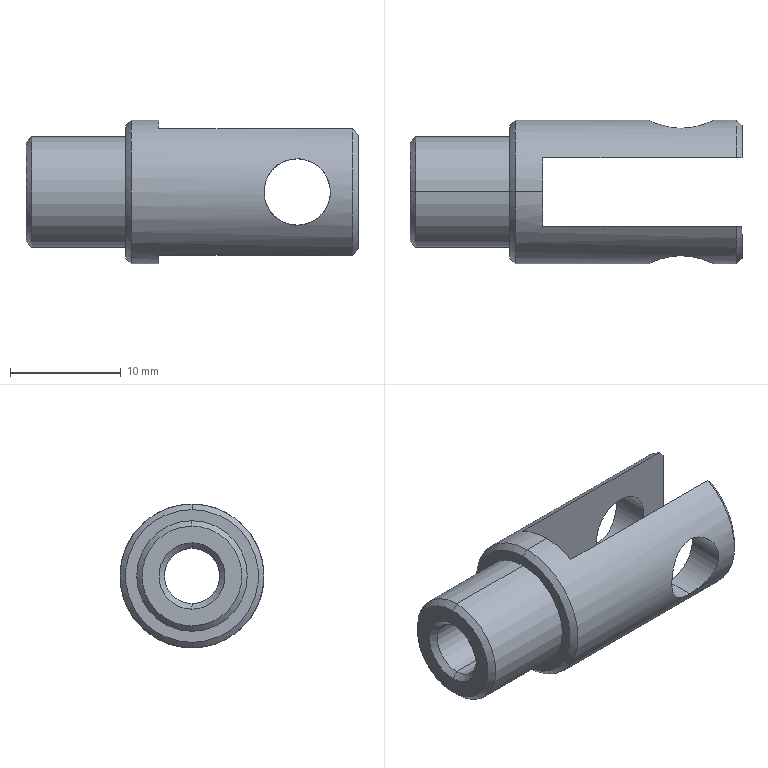Part | STEP file | 101000005929 | 1 solid | 25 faces | box 30 x 13 x 13 mm | volume 1668 mm3 | cylinder 10 | cone 8 | plane 7 | commonest cylinder face diameters 6 x4 5 x2 10 x2 13 x2
STEP:
#1=CARTESIAN_POINT('',(-29.5,0.,-2.5));
#2=VERTEX_POINT('',#1);
#3=CARTESIAN_POINT('',(-29.5,0.,2.5));
#4=VERTEX_POINT('',#3);
#5=CARTESIAN_POINT('',(-29.5,0.,0.));
#6=DIRECTION('',(-1.,0.,0.));
#7=AXIS2_PLACEMENT_3D('',#5,#6,$);
#8=CIRCLE('',#7,2.5);
#9=EDGE_CURVE('',#2,#4,#8,.T.);
#10=ORIENTED_EDGE('',*,*,#9,.F.);
#11=CARTESIAN_POINT('',(-30.,0.,-3.));
#12=VERTEX_POINT('',#11);
#13=CARTESIAN_POINT('',(-353581.641,0.,-353554.641));
#14=DIRECTION('',(-0.7071,0.,-0.7071));
#15=VECTOR('',#14,1.);
#16=LINE('',#13,#15);
#17=EDGE_CURVE('',#2,#12,#16,.T.);
#18=ORIENTED_EDGE('',*,*,#17,.T.);
#19=CARTESIAN_POINT('',(-30.,0.,3.));
#20=VERTEX_POINT('',#19);
#21=CARTESIAN_POINT('',(-30.,0.,0.));
#22=DIRECTION('',(-1.,0.,0.));
#23=AXIS2_PLACEMENT_3D('',#21,#22,$);
#24=CIRCLE('',#23,3.);
#25=EDGE_CURVE('',#20,#12,#24,.F.);
#26=ORIENTED_EDGE('',*,*,#25,.F.);
#27=CARTESIAN_POINT('',(-353581.641,0.,353554.641));
#28=DIRECTION('',(-0.7071,0.,0.7071));
#29=VECTOR('',#28,1.);
#30=LINE('',#27,#29);
#31=EDGE_CURVE('',#4,#20,#30,.T.);
#32=ORIENTED_EDGE('',*,*,#31,.F.);
#33=EDGE_LOOP('',(#10,#18,#26,#32));
#34=FACE_OUTER_BOUND('',#33,.T.);
#35=CARTESIAN_POINT('',(-29.5,0.,0.));
#36=DIRECTION('',(-1.,0.,0.));
#37=DIRECTION('',(0.,0.,-1.));
#38=AXIS2_PLACEMENT_3D('',#35,#36,#37);
#39=CONICAL_SURFACE('',#38,2.5,0.7854);
#40=ADVANCED_FACE('',(#34),#39,.F.);
#41=CARTESIAN_POINT('',(-18.,0.,2.5));
#42=VERTEX_POINT('',#41);
#43=CARTESIAN_POINT('',(-18.,0.,-2.5));
#44=VERTEX_POINT('',#43);
#45=CARTESIAN_POINT('',(-18.,0.,0.));
#46=DIRECTION('',(-1.,0.,0.));
#47=AXIS2_PLACEMENT_3D('',#45,#46,$);
#48=CIRCLE('',#47,2.5);
#49=EDGE_CURVE('',#42,#44,#48,.F.);
#50=ORIENTED_EDGE('',*,*,#49,.T.);
#51=CARTESIAN_POINT('',(-30.,0.,-2.5));
#52=DIRECTION('',(-1.,0.,0.));
#53=VECTOR('',#52,1.);
#54=LINE('',#51,#53);
#55=EDGE_CURVE('',#44,#2,#54,.T.);
#56=ORIENTED_EDGE('',*,*,#55,.T.);
#57=ORIENTED_EDGE('',*,*,#9,.T.);
#58=CARTESIAN_POINT('',(-30.,0.,2.5));
#59=DIRECTION('',(-1.,0.,0.));
#60=VECTOR('',#59,1.);
#61=LINE('',#58,#60);
#62=EDGE_CURVE('',#42,#4,#61,.T.);
#63=ORIENTED_EDGE('',*,*,#62,.F.);
#64=EDGE_LOOP('',(#50,#56,#57,#63));
#65=FACE_OUTER_BOUND('',#64,.T.);
#66=CARTESIAN_POINT('',(-30.,0.,0.));
#67=DIRECTION('',(-1.,0.,0.));
#68=DIRECTION('',(0.,0.,-1.));
#69=AXIS2_PLACEMENT_3D('',#66,#67,#68);
#70=CYLINDRICAL_SURFACE('',#69,2.5);
#71=ADVANCED_FACE('',(#65),#70,.F.);
#72=ORIENTED_EDGE('',*,*,#17,.F.);
#73=CARTESIAN_POINT('',(-29.5,0.,0.));
#74=DIRECTION('',(-1.,0.,0.));
#75=AXIS2_PLACEMENT_3D('',#73,#74,$);
#76=CIRCLE('',#75,2.5);
#77=EDGE_CURVE('',#4,#2,#76,.T.);
#78=ORIENTED_EDGE('',*,*,#77,.F.);
#79=ORIENTED_EDGE('',*,*,#31,.T.);
#80=CARTESIAN_POINT('',(-30.,0.,0.));
#81=DIRECTION('',(-1.,0.,0.));
#82=AXIS2_PLACEMENT_3D('',#80,#81,$);
#83=CIRCLE('',#82,3.);
#84=EDGE_CURVE('',#12,#20,#83,.F.);
#85=ORIENTED_EDGE('',*,*,#84,.F.);
#86=EDGE_LOOP('',(#72,#78,#79,#85));
#87=FACE_OUTER_BOUND('',#86,.T.);
#88=CARTESIAN_POINT('',(-29.5,0.,0.));
#89=DIRECTION('',(-1.,0.,0.));
#90=DIRECTION('',(0.,0.,1.));
#91=AXIS2_PLACEMENT_3D('',#88,#89,#90);
#92=CONICAL_SURFACE('',#91,2.5,0.7854);
#93=ADVANCED_FACE('',(#87),#92,.F.);
#94=CARTESIAN_POINT('',(-30.,0.,-4.5));
#95=VERTEX_POINT('',#94);
#96=CARTESIAN_POINT('',(-30.,0.,4.5));
#97=VERTEX_POINT('',#96);
#98=CARTESIAN_POINT('',(-30.,0.,-4.5));
#99=CARTESIAN_POINT('',(-30.,-0.4157,-4.5));
#100=CARTESIAN_POINT('',(-30.,-0.8314,-4.452));
#101=CARTESIAN_POINT('',(-30.,-1.24,-4.356));
#102=CARTESIAN_POINT('',(-30.,-2.027,-4.071));
#103=CARTESIAN_POINT('',(-30.,-2.728,-3.615));
#104=CARTESIAN_POINT('',(-30.,-3.051,-3.347));
#105=CARTESIAN_POINT('',(-30.,-3.629,-2.742));
#106=CARTESIAN_POINT('',(-30.,-4.053,-2.02));
#107=CARTESIAN_POINT('',(-30.,-4.223,-1.637));
#108=CARTESIAN_POINT('',(-30.,-4.47,-0.8373));
#109=CARTESIAN_POINT('',(-30.,-4.529,-0.002445));
#110=CARTESIAN_POINT('',(-30.,-4.51,0.4166));
#111=CARTESIAN_POINT('',(-30.,-4.375,1.243));
#112=CARTESIAN_POINT('',(-30.,-4.055,2.016));
#113=CARTESIAN_POINT('',(-30.,-3.852,2.383));
#114=CARTESIAN_POINT('',(-30.,-3.363,3.062));
#115=CARTESIAN_POINT('',(-30.,-2.732,3.612));
#116=CARTESIAN_POINT('',(-30.,-2.386,3.849));
#117=CARTESIAN_POINT('',(-30.,-1.719,4.201));
#118=CARTESIAN_POINT('',(-30.,-0.996,4.407));
#119=CARTESIAN_POINT('',(-30.,-0.6666,4.469));
#120=CARTESIAN_POINT('',(-30.,-0.3333,4.5));
#121=CARTESIAN_POINT('',(-30.,0.,4.5));
#122=B_SPLINE_CURVE_WITH_KNOTS('',5,(#98,#99,#100,#101,#102,#103,#104,#105,#106,#107,#108,#109,#110,#111,#112,#113,#114,#115,#116,#117,#118,#119,#120,#121),.UNSPECIFIED.,.F.,.U.,(6,3,3,3,3,3,3,6),(0.,2.939,5.879,8.818,11.757,14.697,17.636,19.993),.UNSPECIFIED.);
#123=EDGE_CURVE('',#95,#97,#122,.T.);
#124=ORIENTED_EDGE('',*,*,#123,.T.);
#125=CARTESIAN_POINT('',(-30.,0.,4.5));
#126=CARTESIAN_POINT('',(-30.,0.4157,4.5));
#127=CARTESIAN_POINT('',(-30.,0.8314,4.452));
#128=CARTESIAN_POINT('',(-30.,1.24,4.356));
#129=CARTESIAN_POINT('',(-30.,2.027,4.071));
#130=CARTESIAN_POINT('',(-30.,2.728,3.615));
#131=CARTESIAN_POINT('',(-30.,3.051,3.347));
#132=CARTESIAN_POINT('',(-30.,3.629,2.742));
#133=CARTESIAN_POINT('',(-30.,4.053,2.02));
#134=CARTESIAN_POINT('',(-30.,4.223,1.637));
#135=CARTESIAN_POINT('',(-30.,4.47,0.8373));
#136=CARTESIAN_POINT('',(-30.,4.529,0.002445));
#137=CARTESIAN_POINT('',(-30.,4.51,-0.4166));
#138=CARTESIAN_POINT('',(-30.,4.375,-1.243));
#139=CARTESIAN_POINT('',(-30.,4.055,-2.016));
#140=CARTESIAN_POINT('',(-30.,3.852,-2.383));
#141=CARTESIAN_POINT('',(-30.,3.363,-3.062));
#142=CARTESIAN_POINT('',(-30.,2.732,-3.612));
#143=CARTESIAN_POINT('',(-30.,2.386,-3.849));
#144=CARTESIAN_POINT('',(-30.,1.719,-4.201));
#145=CARTESIAN_POINT('',(-30.,0.996,-4.407));
#146=CARTESIAN_POINT('',(-30.,0.6666,-4.469));
#147=CARTESIAN_POINT('',(-30.,0.3333,-4.5));
#148=CARTESIAN_POINT('',(-30.,0.,-4.5));
#149=B_SPLINE_CURVE_WITH_KNOTS('',5,(#125,#126,#127,#128,#129,#130,#131,#132,#133,#134,#135,#136,#137,#138,#139,#140,#141,#142,#143,#144,#145,#146,#147,#148),.UNSPECIFIED.,.F.,.U.,(6,3,3,3,3,3,3,6),(0.,2.939,5.879,8.818,11.757,14.697,17.636,19.993),.UNSPECIFIED.);
#150=EDGE_CURVE('',#97,#95,#149,.T.);
#151=ORIENTED_EDGE('',*,*,#150,.T.);
#152=EDGE_LOOP('',(#124,#151));
#153=FACE_OUTER_BOUND('',#152,.T.);
#154=ORIENTED_EDGE('',*,*,#25,.T.);
#155=ORIENTED_EDGE('',*,*,#84,.T.);
#156=EDGE_LOOP('',(#154,#155));
#157=FACE_BOUND('',#156,.T.);
#158=CARTESIAN_POINT('',(-30.,0.,0.));
#159=DIRECTION('',(1.,0.,0.));
#160=DIRECTION('',(0.,0.,-1.));
#161=AXIS2_PLACEMENT_3D('',#158,#159,#160);
#162=PLANE('',#161);
#163=ADVANCED_FACE('',(#153,#157),#162,.F.);
#164=CARTESIAN_POINT('',(-18.,3.1,5.713));
#165=VERTEX_POINT('',#164);
#166=CARTESIAN_POINT('',(-18.,3.1,-5.713));
#167=VERTEX_POINT('',#166);
#168=CARTESIAN_POINT('',(-18.,3.1,0.));
#169=DIRECTION('',(0.,0.,-1.));
#170=VECTOR('',#169,1.);
#171=LINE('',#168,#170);
#172=EDGE_CURVE('',#165,#167,#171,.T.);
#173=ORIENTED_EDGE('',*,*,#172,.F.);
#174=CARTESIAN_POINT('',(-18.,0.,6.5));
#175=VERTEX_POINT('',#174);
#176=CARTESIAN_POINT('',(-18.,-0.000000001,0.000000005));
#177=DIRECTION('',(1.,0.,0.));
#178=AXIS2_PLACEMENT_3D('',#176,#177,$);
#179=CIRCLE('',#178,6.5);
#180=EDGE_CURVE('',#165,#175,#179,.T.);
#181=ORIENTED_EDGE('',*,*,#180,.T.);
#182=CARTESIAN_POINT('',(-18.,-3.1,5.713));
#183=VERTEX_POINT('',#182);
#184=CARTESIAN_POINT('',(-18.,0.000000002,0.000000005));
#185=DIRECTION('',(1.,0.,0.));
#186=AXIS2_PLACEMENT_3D('',#184,#185,$);
#187=CIRCLE('',#186,6.5);
#188=EDGE_CURVE('',#175,#183,#187,.T.);
#189=ORIENTED_EDGE('',*,*,#188,.T.);
#190=CARTESIAN_POINT('',(-18.,-3.1,-5.713));
#191=VERTEX_POINT('',#190);
#192=CARTESIAN_POINT('',(-18.,-3.1,0.));
#193=DIRECTION('',(0.,0.,-1.));
#194=VECTOR('',#193,1.);
#195=LINE('',#192,#194);
#196=EDGE_CURVE('',#183,#191,#195,.T.);
#197=ORIENTED_EDGE('',*,*,#196,.T.);
#198=CARTESIAN_POINT('',(-18.,0.,-6.5));
#199=VERTEX_POINT('',#198);
#200=CARTESIAN_POINT('',(-18.,-0.000000009,-0.000000034));
#201=DIRECTION('',(1.,0.,0.));
#202=AXIS2_PLACEMENT_3D('',#200,#201,$);
#203=CIRCLE('',#202,6.5);
#204=EDGE_CURVE('',#191,#199,#203,.T.);
#205=ORIENTED_EDGE('',*,*,#204,.T.);
#206=CARTESIAN_POINT('',(-18.,0.00000001,-0.000000034));
#207=DIRECTION('',(1.,0.,0.));
#208=AXIS2_PLACEMENT_3D('',#206,#207,$);
#209=CIRCLE('',#208,6.5);
#210=EDGE_CURVE('',#199,#167,#209,.T.);
#211=ORIENTED_EDGE('',*,*,#210,.T.);
#212=EDGE_LOOP('',(#173,#181,#189,#197,#205,#211));
#213=FACE_OUTER_BOUND('',#212,.T.);
#214=ORIENTED_EDGE('',*,*,#49,.F.);
#215=CARTESIAN_POINT('',(-18.,0.,0.000000001));
#216=DIRECTION('',(1.,0.,0.));
#217=AXIS2_PLACEMENT_3D('',#215,#216,$);
#218=CIRCLE('',#217,2.5);
#219=EDGE_CURVE('',#44,#42,#218,.T.);
#220=ORIENTED_EDGE('',*,*,#219,.F.);
#221=EDGE_LOOP('',(#214,#220));
#222=FACE_BOUND('',#221,.T.);
#223=CARTESIAN_POINT('',(-18.,3.1,50.232));
#224=DIRECTION('',(1.,0.,0.));
#225=DIRECTION('',(0.,1.,0.));
#226=AXIS2_PLACEMENT_3D('',#223,#224,#225);
#227=PLANE('',#226);
#228=ADVANCED_FACE('',(#213,#222),#227,.T.);
#229=ORIENTED_EDGE('',*,*,#55,.F.);
#230=ORIENTED_EDGE('',*,*,#219,.T.);
#231=ORIENTED_EDGE('',*,*,#62,.T.);
#232=ORIENTED_EDGE('',*,*,#77,.T.);
#233=EDGE_LOOP('',(#229,#230,#231,#232));
#234=FACE_OUTER_BOUND('',#233,.T.);
#235=CARTESIAN_POINT('',(-30.,0.,0.));
#236=DIRECTION('',(-1.,0.,0.));
#237=DIRECTION('',(0.,0.,1.));
#238=AXIS2_PLACEMENT_3D('',#235,#236,#237);
#239=CYLINDRICAL_SURFACE('',#238,2.5);
#240=ADVANCED_FACE('',(#234),#239,.F.);
#241=CARTESIAN_POINT('',(-29.5,0.,5.));
#242=VERTEX_POINT('',#241);
#243=CARTESIAN_POINT('',(353521.141,0.,353555.641));
#244=DIRECTION('',(0.7071,0.,0.7071));
#245=VECTOR('',#244,1.);
#246=LINE('',#243,#245);
#247=EDGE_CURVE('',#97,#242,#246,.T.);
#248=ORIENTED_EDGE('',*,*,#247,.F.);
#249=ORIENTED_EDGE('',*,*,#123,.F.);
#250=CARTESIAN_POINT('',(-29.5,0.,-5.));
#251=VERTEX_POINT('',#250);
#252=CARTESIAN_POINT('',(353521.141,0.,-353555.641));
#253=DIRECTION('',(0.7071,0.,-0.7071));
#254=VECTOR('',#253,1.);
#255=LINE('',#252,#254);
#256=EDGE_CURVE('',#95,#251,#255,.T.);
#257=ORIENTED_EDGE('',*,*,#256,.T.);
#258=CARTESIAN_POINT('',(-29.5,0.,0.));
#259=DIRECTION('',(1.,0.,0.));
#260=AXIS2_PLACEMENT_3D('',#258,#259,$);
#261=CIRCLE('',#260,5.);
#262=EDGE_CURVE('',#242,#251,#261,.T.);
#263=ORIENTED_EDGE('',*,*,#262,.F.);
#264=EDGE_LOOP('',(#248,#249,#257,#263));
#265=FACE_OUTER_BOUND('',#264,.T.);
#266=CARTESIAN_POINT('',(-30.,0.,0.));
#267=DIRECTION('',(1.,0.,0.));
#268=DIRECTION('',(0.,0.,1.));
#269=AXIS2_PLACEMENT_3D('',#266,#267,#268);
#270=CONICAL_SURFACE('',#269,4.5,0.7854);
#271=ADVANCED_FACE('',(#265),#270,.T.);
#272=ORIENTED_EDGE('',*,*,#150,.F.);
#273=ORIENTED_EDGE('',*,*,#247,.T.);
#274=CARTESIAN_POINT('',(-29.5,0.,0.));
#275=DIRECTION('',(1.,0.,0.));
#276=AXIS2_PLACEMENT_3D('',#274,#275,$);
#277=CIRCLE('',#276,5.);
#278=EDGE_CURVE('',#251,#242,#277,.T.);
#279=ORIENTED_EDGE('',*,*,#278,.F.);
#280=ORIENTED_EDGE('',*,*,#256,.F.);
#281=EDGE_LOOP('',(#272,#273,#279,#280));
#282=FACE_OUTER_BOUND('',#281,.T.);
#283=CARTESIAN_POINT('',(-30.,0.,0.));
#284=DIRECTION('',(1.,0.,0.));
#285=DIRECTION('',(0.,0.,-1.));
#286=AXIS2_PLACEMENT_3D('',#283,#284,#285);
#287=CONICAL_SURFACE('',#286,4.5,0.7854);
#288=ADVANCED_FACE('',(#282),#287,.T.);
#289=CARTESIAN_POINT('',(-0.5,3.1,-5.713));
#290=VERTEX_POINT('',#289);
#291=CARTESIAN_POINT('',(-9.25,3.1,-5.713));
#292=DIRECTION('',(1.,0.,0.));
#293=VECTOR('',#292,1.);
#294=LINE('',#291,#293);
#295=EDGE_CURVE('',#167,#290,#294,.T.);
#296=ORIENTED_EDGE('',*,*,#295,.T.);
#297=CARTESIAN_POINT('',(0.,3.1,-5.137));
#298=VERTEX_POINT('',#297);
#299=CARTESIAN_POINT('',(-0.5,3.1,-5.713));
#300=CARTESIAN_POINT('',(-0.3993,3.1,-5.599));
#301=CARTESIAN_POINT('',(-0.2989,3.1,-5.484));
#302=CARTESIAN_POINT('',(-0.1989,3.1,-5.369));
#303=CARTESIAN_POINT('',(-0.09922,3.1,-5.253));
#304=CARTESIAN_POINT('',(0.,3.1,-5.137));
#305=B_SPLINE_CURVE_WITH_KNOTS('',5,(#299,#300,#301,#302,#303,#304),.UNSPECIFIED.,.F.,.U.,(6,6),(0.,1.079),.UNSPECIFIED.);
#306=EDGE_CURVE('',#290,#298,#305,.T.);
#307=ORIENTED_EDGE('',*,*,#306,.T.);
#308=CARTESIAN_POINT('',(0.,3.1,5.137));
#309=VERTEX_POINT('',#308);
#310=CARTESIAN_POINT('',(0.,3.1,0.));
#311=DIRECTION('',(0.,0.,1.));
#312=VECTOR('',#311,1.);
#313=LINE('',#310,#312);
#314=EDGE_CURVE('',#298,#309,#313,.T.);
#315=ORIENTED_EDGE('',*,*,#314,.T.);
#316=CARTESIAN_POINT('',(-0.5,3.1,5.713));
#317=VERTEX_POINT('',#316);
#318=CARTESIAN_POINT('',(0.,3.1,5.137));
#319=CARTESIAN_POINT('',(-0.09922,3.1,5.253));
#320=CARTESIAN_POINT('',(-0.1989,3.1,5.369));
#321=CARTESIAN_POINT('',(-0.2989,3.1,5.484));
#322=CARTESIAN_POINT('',(-0.3993,3.1,5.599));
#323=CARTESIAN_POINT('',(-0.5,3.1,5.713));
#324=B_SPLINE_CURVE_WITH_KNOTS('',5,(#318,#319,#320,#321,#322,#323),.UNSPECIFIED.,.F.,.U.,(6,6),(0.,1.079),.UNSPECIFIED.);
#325=EDGE_CURVE('',#309,#317,#324,.T.);
#326=ORIENTED_EDGE('',*,*,#325,.T.);
#327=CARTESIAN_POINT('',(-9.25,3.1,5.713));
#328=DIRECTION('',(-1.,0.,0.));
#329=VECTOR('',#328,1.);
#330=LINE('',#327,#329);
#331=EDGE_CURVE('',#317,#165,#330,.T.);
#332=ORIENTED_EDGE('',*,*,#331,.T.);
#333=ORIENTED_EDGE('',*,*,#172,.T.);
#334=EDGE_LOOP('',(#296,#307,#315,#326,#332,#333));
#335=FACE_OUTER_BOUND('',#334,.T.);
#336=CARTESIAN_POINT('',(-5.5,3.1,-3.));
#337=VERTEX_POINT('',#336);
#338=CARTESIAN_POINT('',(-5.5,3.1,3.));
#339=VERTEX_POINT('',#338);
#340=CARTESIAN_POINT('',(-5.5,3.1,-3.));
#341=CARTESIAN_POINT('',(-5.839,3.1,-3.));
#342=CARTESIAN_POINT('',(-6.179,3.1,-2.952));
#343=CARTESIAN_POINT('',(-6.509,3.1,-2.856));
#344=CARTESIAN_POINT('',(-7.134,3.1,-2.573));
#345=CARTESIAN_POINT('',(-7.655,3.1,-2.128));
#346=CARTESIAN_POINT('',(-7.883,3.1,-1.87));
#347=CARTESIAN_POINT('',(-8.258,3.1,-1.297));
#348=CARTESIAN_POINT('',(-8.46,3.1,-0.6415));
#349=CARTESIAN_POINT('',(-8.514,3.1,-0.3017));
#350=CARTESIAN_POINT('',(-8.524,3.1,0.3838));
#351=CARTESIAN_POINT('',(-8.343,3.1,1.045));
#352=CARTESIAN_POINT('',(-8.206,3.1,1.361));
#353=CARTESIAN_POINT('',(-7.847,3.1,1.945));
#354=CARTESIAN_POINT('',(-7.34,3.1,2.406));
#355=CARTESIAN_POINT('',(-7.055,3.1,2.599));
#356=CARTESIAN_POINT('',(-6.577,3.1,2.833));
#357=CARTESIAN_POINT('',(-6.062,3.1,2.956));
#358=CARTESIAN_POINT('',(-5.876,3.1,2.985));
#359=CARTESIAN_POINT('',(-5.688,3.1,3.));
#360=CARTESIAN_POINT('',(-5.5,3.1,3.));
#361=B_SPLINE_CURVE_WITH_KNOTS('',5,(#340,#341,#342,#343,#344,#345,#346,#347,#348,#349,#350,#351,#352,#353,#354,#355,#356,#357,#358,#359,#360),.UNSPECIFIED.,.F.,.U.,(6,3,3,3,3,3,6),(0.,2.4,4.8,7.2,9.6,12.,13.328),.UNSPECIFIED.);
#362=EDGE_CURVE('',#337,#339,#361,.T.);
#363=ORIENTED_EDGE('',*,*,#362,.T.);
#364=CARTESIAN_POINT('',(-5.5,3.1,3.));
#365=CARTESIAN_POINT('',(-5.161,3.1,3.));
#366=CARTESIAN_POINT('',(-4.821,3.1,2.952));
#367=CARTESIAN_POINT('',(-4.491,3.1,2.856));
#368=CARTESIAN_POINT('',(-3.866,3.1,2.573));
#369=CARTESIAN_POINT('',(-3.345,3.1,2.128));
#370=CARTESIAN_POINT('',(-3.117,3.1,1.87));
#371=CARTESIAN_POINT('',(-2.742,3.1,1.297));
#372=CARTESIAN_POINT('',(-2.54,3.1,0.6415));
#373=CARTESIAN_POINT('',(-2.486,3.1,0.3017));
#374=CARTESIAN_POINT('',(-2.476,3.1,-0.3838));
#375=CARTESIAN_POINT('',(-2.657,3.1,-1.045));
#376=CARTESIAN_POINT('',(-2.794,3.1,-1.361));
#377=CARTESIAN_POINT('',(-3.153,3.1,-1.945));
#378=CARTESIAN_POINT('',(-3.66,3.1,-2.406));
#379=CARTESIAN_POINT('',(-3.945,3.1,-2.599));
#380=CARTESIAN_POINT('',(-4.423,3.1,-2.833));
#381=CARTESIAN_POINT('',(-4.938,3.1,-2.956));
#382=CARTESIAN_POINT('',(-5.124,3.1,-2.985));
#383=CARTESIAN_POINT('',(-5.312,3.1,-3.));
#384=CARTESIAN_POINT('',(-5.5,3.1,-3.));
#385=B_SPLINE_CURVE_WITH_KNOTS('',5,(#364,#365,#366,#367,#368,#369,#370,#371,#372,#373,#374,#375,#376,#377,#378,#379,#380,#381,#382,#383,#384),.UNSPECIFIED.,.F.,.U.,(6,3,3,3,3,3,6),(0.,2.4,4.8,7.2,9.6,12.,13.328),.UNSPECIFIED.);
#386=EDGE_CURVE('',#339,#337,#385,.T.);
#387=ORIENTED_EDGE('',*,*,#386,.T.);
#388=EDGE_LOOP('',(#363,#387));
#389=FACE_BOUND('',#388,.T.);
#390=CARTESIAN_POINT('',(0.,3.1,50.232));
#391=DIRECTION('',(0.,-1.,0.));
#392=DIRECTION('',(1.,0.,0.));
#393=AXIS2_PLACEMENT_3D('',#390,#391,#392);
#394=PLANE('',#393);
#395=ADVANCED_FACE('',(#335,#389),#394,.T.);
#396=ORIENTED_EDGE('',*,*,#210,.F.);
#397=CARTESIAN_POINT('',(-20.5,0.,-6.5));
#398=VERTEX_POINT('',#397);
#399=CARTESIAN_POINT('',(-30.,0.,-6.5));
#400=DIRECTION('',(-1.,0.,0.));
#401=VECTOR('',#400,1.);
#402=LINE('',#399,#401);
#403=EDGE_CURVE('',#199,#398,#402,.T.);
#404=ORIENTED_EDGE('',*,*,#403,.T.);
#405=CARTESIAN_POINT('',(-20.5,0.,6.5));
#406=VERTEX_POINT('',#405);
#407=CARTESIAN_POINT('',(-20.5,0.,0.));
#408=DIRECTION('',(-1.,0.,0.));
#409=AXIS2_PLACEMENT_3D('',#407,#408,$);
#410=CIRCLE('',#409,6.5);
#411=EDGE_CURVE('',#398,#406,#410,.F.);
#412=ORIENTED_EDGE('',*,*,#411,.T.);
#413=CARTESIAN_POINT('',(-30.,0.,6.5));
#414=DIRECTION('',(-1.,0.,0.));
#415=VECTOR('',#414,1.);
#416=LINE('',#413,#415);
#417=EDGE_CURVE('',#175,#406,#416,.T.);
#418=ORIENTED_EDGE('',*,*,#417,.F.);
#419=ORIENTED_EDGE('',*,*,#180,.F.);
#420=ORIENTED_EDGE('',*,*,#331,.F.);
#421=CARTESIAN_POINT('',(-0.5,0.,0.));
#422=DIRECTION('',(-1.,0.,0.));
#423=AXIS2_PLACEMENT_3D('',#421,#422,$);
#424=CIRCLE('',#423,6.5);
#425=EDGE_CURVE('',#317,#290,#424,.T.);
#426=ORIENTED_EDGE('',*,*,#425,.T.);
#427=ORIENTED_EDGE('',*,*,#295,.F.);
#428=EDGE_LOOP('',(#396,#404,#412,#418,#419,#420,#426,#427));
#429=FACE_OUTER_BOUND('',#428,.T.);
#430=CARTESIAN_POINT('',(-5.5,5.766,-3.));
#431=VERTEX_POINT('',#430);
#432=CARTESIAN_POINT('',(-5.5,5.766,3.));
#433=VERTEX_POINT('',#432);
#434=CARTESIAN_POINT('',(-5.5,5.766,-3.));
#435=CARTESIAN_POINT('',(-5.829,5.766,-3.));
#436=CARTESIAN_POINT('',(-6.152,5.789,-2.956));
#437=CARTESIAN_POINT('',(-6.469,5.835,-2.867));
#438=CARTESIAN_POINT('',(-7.002,5.947,-2.636));
#439=CARTESIAN_POINT('',(-7.461,6.086,-2.291));
#440=CARTESIAN_POINT('',(-7.645,6.149,-2.121));
#441=CARTESIAN_POINT('',(-8.024,6.29,-1.684));
#442=CARTESIAN_POINT('',(-8.293,6.405,-1.167));
#443=CARTESIAN_POINT('',(-8.404,6.456,-0.8542));
#444=CARTESIAN_POINT('',(-8.538,6.517,-0.2095));
#445=CARTESIAN_POINT('',(-8.493,6.497,0.4514));
#446=CARTESIAN_POINT('',(-8.425,6.465,0.7775));
#447=CARTESIAN_POINT('',(-8.229,6.377,1.326));
#448=CARTESIAN_POINT('',(-7.916,6.25,1.805));
#449=CARTESIAN_POINT('',(-7.755,6.188,2.002));
#450=CARTESIAN_POINT('',(-7.46,6.085,2.296));
#451=CARTESIAN_POINT('',(-7.118,5.987,2.534));
#452=CARTESIAN_POINT('',(-6.974,5.949,2.621));
#453=CARTESIAN_POINT('',(-6.614,5.866,2.805));
#454=CARTESIAN_POINT('',(-6.223,5.805,2.926));
#455=CARTESIAN_POINT('',(-5.984,5.779,2.975));
#456=CARTESIAN_POINT('',(-5.741,5.766,3.));
#457=CARTESIAN_POINT('',(-5.5,5.766,3.));
#458=B_SPLINE_CURVE_WITH_KNOTS('',5,(#434,#435,#436,#437,#438,#439,#440,#441,#442,#443,#444,#445,#446,#447,#448,#449,#450,#451,#452,#453,#454,#455,#456,#457),.UNSPECIFIED.,.F.,.U.,(6,3,3,3,3,3,3,6),(0.,2.313,4.158,6.496,8.8,10.625,11.825,13.541),.UNSPECIFIED.);
#459=EDGE_CURVE('',#431,#433,#458,.T.);
#460=ORIENTED_EDGE('',*,*,#459,.F.);
#461=CARTESIAN_POINT('',(-5.5,5.766,3.));
#462=CARTESIAN_POINT('',(-5.089,5.766,3.));
#463=CARTESIAN_POINT('',(-4.674,5.804,2.928));
#464=CARTESIAN_POINT('',(-4.284,5.877,2.788));
#465=CARTESIAN_POINT('',(-3.78,6.008,2.503));
#466=CARTESIAN_POINT('',(-3.363,6.148,2.115));
#467=CARTESIAN_POINT('',(-3.248,6.189,1.992));
#468=CARTESIAN_POINT('',(-3.039,6.268,1.735));
#469=CARTESIAN_POINT('',(-2.866,6.339,1.449));
#470=CARTESIAN_POINT('',(-2.789,6.371,1.301));
#471=CARTESIAN_POINT('',(-2.66,6.427,1.001));
#472=CARTESIAN_POINT('',(-2.573,6.467,0.6849));
#473=CARTESIAN_POINT('',(-2.54,6.482,0.5261));
#474=CARTESIAN_POINT('',(-2.485,6.507,0.1234));
#475=CARTESIAN_POINT('',(-2.498,6.501,-0.285));
#476=CARTESIAN_POINT('',(-2.532,6.485,-0.5294));
#477=CARTESIAN_POINT('',(-2.67,6.422,-1.097));
#478=CARTESIAN_POINT('',(-2.936,6.308,-1.612));
#479=CARTESIAN_POINT('',(-3.131,6.23,-1.884));
#480=CARTESIAN_POINT('',(-3.635,6.045,-2.421));
#481=CARTESIAN_POINT('',(-4.284,5.877,-2.787));
#482=CARTESIAN_POINT('',(-4.673,5.804,-2.928));
#483=CARTESIAN_POINT('',(-5.085,5.766,-3.));
#484=CARTESIAN_POINT('',(-5.5,5.766,-3.));
#485=B_SPLINE_CURVE_WITH_KNOTS('',5,(#461,#462,#463,#464,#465,#466,#467,#468,#469,#470,#471,#472,#473,#474,#475,#476,#477,#478,#479,#480,#481,#482,#483,#484),.UNSPECIFIED.,.F.,.U.,(6,3,3,3,3,3,3,6),(0.,2.915,4.139,5.326,6.479,8.198,10.612,13.532),.UNSPECIFIED.);
#486=EDGE_CURVE('',#433,#431,#485,.T.);
#487=ORIENTED_EDGE('',*,*,#486,.F.);
#488=EDGE_LOOP('',(#460,#487));
#489=FACE_BOUND('',#488,.T.);
#490=CARTESIAN_POINT('',(-30.,0.,0.));
#491=DIRECTION('',(-1.,0.,0.));
#492=DIRECTION('',(0.,0.,1.));
#493=AXIS2_PLACEMENT_3D('',#490,#491,#492);
#494=CYLINDRICAL_SURFACE('',#493,6.5);
#495=ADVANCED_FACE('',(#429,#489),#494,.T.);
#496=ORIENTED_EDGE('',*,*,#403,.F.);
#497=ORIENTED_EDGE('',*,*,#204,.F.);
#498=CARTESIAN_POINT('',(-0.5,-3.1,-5.713));
#499=VERTEX_POINT('',#498);
#500=CARTESIAN_POINT('',(-30.,-3.1,-5.713));
#501=DIRECTION('',(-1.,0.,0.));
#502=VECTOR('',#501,1.);
#503=LINE('',#500,#502);
#504=EDGE_CURVE('',#499,#191,#503,.T.);
#505=ORIENTED_EDGE('',*,*,#504,.F.);
#506=CARTESIAN_POINT('',(-0.5,-3.1,5.713));
#507=VERTEX_POINT('',#506);
#508=CARTESIAN_POINT('',(-0.5,0.,0.));
#509=DIRECTION('',(-1.,0.,0.));
#510=AXIS2_PLACEMENT_3D('',#508,#509,$);
#511=CIRCLE('',#510,6.5);
#512=EDGE_CURVE('',#499,#507,#511,.T.);
#513=ORIENTED_EDGE('',*,*,#512,.T.);
#514=CARTESIAN_POINT('',(-30.,-3.1,5.713));
#515=DIRECTION('',(-1.,0.,0.));
#516=VECTOR('',#515,1.);
#517=LINE('',#514,#516);
#518=EDGE_CURVE('',#183,#507,#517,.F.);
#519=ORIENTED_EDGE('',*,*,#518,.F.);
#520=ORIENTED_EDGE('',*,*,#188,.F.);
#521=ORIENTED_EDGE('',*,*,#417,.T.);
#522=CARTESIAN_POINT('',(-20.5,0.,0.));
#523=DIRECTION('',(-1.,0.,0.));
#524=AXIS2_PLACEMENT_3D('',#522,#523,$);
#525=CIRCLE('',#524,6.5);
#526=EDGE_CURVE('',#406,#398,#525,.F.);
#527=ORIENTED_EDGE('',*,*,#526,.T.);
#528=EDGE_LOOP('',(#496,#497,#505,#513,#519,#520,#521,#527));
#529=FACE_OUTER_BOUND('',#528,.T.);
#530=CARTESIAN_POINT('',(-5.5,-5.766,-3.));
#531=VERTEX_POINT('',#530);
#532=CARTESIAN_POINT('',(-5.5,-5.766,3.));
#533=VERTEX_POINT('',#532);
#534=CARTESIAN_POINT('',(-5.5,-5.766,-3.));
#535=CARTESIAN_POINT('',(-5.171,-5.766,-3.));
#536=CARTESIAN_POINT('',(-4.848,-5.789,-2.956));
#537=CARTESIAN_POINT('',(-4.531,-5.835,-2.867));
#538=CARTESIAN_POINT('',(-3.998,-5.947,-2.636));
#539=CARTESIAN_POINT('',(-3.539,-6.086,-2.291));
#540=CARTESIAN_POINT('',(-3.355,-6.149,-2.121));
#541=CARTESIAN_POINT('',(-2.976,-6.29,-1.684));
#542=CARTESIAN_POINT('',(-2.707,-6.405,-1.167));
#543=CARTESIAN_POINT('',(-2.596,-6.456,-0.8542));
#544=CARTESIAN_POINT('',(-2.462,-6.517,-0.2095));
#545=CARTESIAN_POINT('',(-2.507,-6.497,0.4514));
#546=CARTESIAN_POINT('',(-2.575,-6.465,0.7775));
#547=CARTESIAN_POINT('',(-2.771,-6.377,1.326));
#548=CARTESIAN_POINT('',(-3.084,-6.25,1.805));
#549=CARTESIAN_POINT('',(-3.245,-6.188,2.002));
#550=CARTESIAN_POINT('',(-3.54,-6.085,2.296));
#551=CARTESIAN_POINT('',(-3.882,-5.987,2.534));
#552=CARTESIAN_POINT('',(-4.026,-5.949,2.621));
#553=CARTESIAN_POINT('',(-4.386,-5.866,2.805));
#554=CARTESIAN_POINT('',(-4.777,-5.805,2.926));
#555=CARTESIAN_POINT('',(-5.016,-5.779,2.975));
#556=CARTESIAN_POINT('',(-5.259,-5.766,3.));
#557=CARTESIAN_POINT('',(-5.5,-5.766,3.));
#558=B_SPLINE_CURVE_WITH_KNOTS('',5,(#534,#535,#536,#537,#538,#539,#540,#541,#542,#543,#544,#545,#546,#547,#548,#549,#550,#551,#552,#553,#554,#555,#556,#557),.UNSPECIFIED.,.F.,.U.,(6,3,3,3,3,3,3,6),(0.,2.313,4.158,6.496,8.8,10.625,11.825,13.541),.UNSPECIFIED.);
#559=EDGE_CURVE('',#531,#533,#558,.T.);
#560=ORIENTED_EDGE('',*,*,#559,.F.);
#561=CARTESIAN_POINT('',(-5.5,-5.766,3.));
#562=CARTESIAN_POINT('',(-5.911,-5.766,3.));
#563=CARTESIAN_POINT('',(-6.326,-5.804,2.928));
#564=CARTESIAN_POINT('',(-6.716,-5.877,2.788));
#565=CARTESIAN_POINT('',(-7.22,-6.008,2.503));
#566=CARTESIAN_POINT('',(-7.637,-6.148,2.115));
#567=CARTESIAN_POINT('',(-7.752,-6.189,1.992));
#568=CARTESIAN_POINT('',(-7.961,-6.268,1.735));
#569=CARTESIAN_POINT('',(-8.134,-6.339,1.449));
#570=CARTESIAN_POINT('',(-8.211,-6.371,1.301));
#571=CARTESIAN_POINT('',(-8.34,-6.427,1.001));
#572=CARTESIAN_POINT('',(-8.427,-6.467,0.6849));
#573=CARTESIAN_POINT('',(-8.46,-6.482,0.5261));
#574=CARTESIAN_POINT('',(-8.515,-6.507,0.1234));
#575=CARTESIAN_POINT('',(-8.502,-6.501,-0.285));
#576=CARTESIAN_POINT('',(-8.468,-6.485,-0.5294));
#577=CARTESIAN_POINT('',(-8.33,-6.422,-1.097));
#578=CARTESIAN_POINT('',(-8.064,-6.308,-1.612));
#579=CARTESIAN_POINT('',(-7.869,-6.23,-1.884));
#580=CARTESIAN_POINT('',(-7.365,-6.045,-2.421));
#581=CARTESIAN_POINT('',(-6.716,-5.877,-2.787));
#582=CARTESIAN_POINT('',(-6.327,-5.804,-2.928));
#583=CARTESIAN_POINT('',(-5.915,-5.766,-3.));
#584=CARTESIAN_POINT('',(-5.5,-5.766,-3.));
#585=B_SPLINE_CURVE_WITH_KNOTS('',5,(#561,#562,#563,#564,#565,#566,#567,#568,#569,#570,#571,#572,#573,#574,#575,#576,#577,#578,#579,#580,#581,#582,#583,#584),.UNSPECIFIED.,.F.,.U.,(6,3,3,3,3,3,3,6),(0.,2.915,4.139,5.326,6.479,8.198,10.612,13.532),.UNSPECIFIED.);
#586=EDGE_CURVE('',#533,#531,#585,.T.);
#587=ORIENTED_EDGE('',*,*,#586,.F.);
#588=EDGE_LOOP('',(#560,#587));
#589=FACE_BOUND('',#588,.T.);
#590=CARTESIAN_POINT('',(-30.,0.,0.));
#591=DIRECTION('',(-1.,0.,0.));
#592=DIRECTION('',(0.,0.,-1.));
#593=AXIS2_PLACEMENT_3D('',#590,#591,#592);
#594=CYLINDRICAL_SURFACE('',#593,6.5);
#595=ADVANCED_FACE('',(#529,#589),#594,.T.);
#596=ORIENTED_EDGE('',*,*,#518,.T.);
#597=CARTESIAN_POINT('',(0.,-3.1,5.137));
#598=VERTEX_POINT('',#597);
#599=CARTESIAN_POINT('',(-0.5,-3.1,5.713));
#600=CARTESIAN_POINT('',(-0.3993,-3.1,5.599));
#601=CARTESIAN_POINT('',(-0.2989,-3.1,5.484));
#602=CARTESIAN_POINT('',(-0.1989,-3.1,5.369));
#603=CARTESIAN_POINT('',(-0.09922,-3.1,5.253));
#604=CARTESIAN_POINT('',(0.,-3.1,5.137));
#605=B_SPLINE_CURVE_WITH_KNOTS('',5,(#599,#600,#601,#602,#603,#604),.UNSPECIFIED.,.F.,.U.,(6,6),(0.,1.079),.UNSPECIFIED.);
#606=EDGE_CURVE('',#507,#598,#605,.T.);
#607=ORIENTED_EDGE('',*,*,#606,.T.);
#608=CARTESIAN_POINT('',(0.,-3.1,-5.137));
#609=VERTEX_POINT('',#608);
#610=CARTESIAN_POINT('',(0.,-3.1,0.));
#611=DIRECTION('',(0.,0.,-1.));
#612=VECTOR('',#611,1.);
#613=LINE('',#610,#612);
#614=EDGE_CURVE('',#598,#609,#613,.T.);
#615=ORIENTED_EDGE('',*,*,#614,.T.);
#616=CARTESIAN_POINT('',(0.,-3.1,-5.137));
#617=CARTESIAN_POINT('',(-0.09922,-3.1,-5.253));
#618=CARTESIAN_POINT('',(-0.1989,-3.1,-5.369));
#619=CARTESIAN_POINT('',(-0.2989,-3.1,-5.484));
#620=CARTESIAN_POINT('',(-0.3993,-3.1,-5.599));
#621=CARTESIAN_POINT('',(-0.5,-3.1,-5.713));
#622=B_SPLINE_CURVE_WITH_KNOTS('',5,(#616,#617,#618,#619,#620,#621),.UNSPECIFIED.,.F.,.U.,(6,6),(0.,1.079),.UNSPECIFIED.);
#623=EDGE_CURVE('',#609,#499,#622,.T.);
#624=ORIENTED_EDGE('',*,*,#623,.T.);
#625=ORIENTED_EDGE('',*,*,#504,.T.);
#626=ORIENTED_EDGE('',*,*,#196,.F.);
#627=EDGE_LOOP('',(#596,#607,#615,#624,#625,#626));
#628=FACE_OUTER_BOUND('',#627,.T.);
#629=CARTESIAN_POINT('',(-5.5,-3.1,-3.));
#630=VERTEX_POINT('',#629);
#631=CARTESIAN_POINT('',(-5.5,-3.1,3.));
#632=VERTEX_POINT('',#631);
#633=CARTESIAN_POINT('',(-5.5,-3.1,-3.));
#634=CARTESIAN_POINT('',(-5.161,-3.1,-3.));
#635=CARTESIAN_POINT('',(-4.821,-3.1,-2.952));
#636=CARTESIAN_POINT('',(-4.491,-3.1,-2.856));
#637=CARTESIAN_POINT('',(-3.866,-3.1,-2.573));
#638=CARTESIAN_POINT('',(-3.345,-3.1,-2.128));
#639=CARTESIAN_POINT('',(-3.117,-3.1,-1.87));
#640=CARTESIAN_POINT('',(-2.742,-3.1,-1.297));
#641=CARTESIAN_POINT('',(-2.54,-3.1,-0.6415));
#642=CARTESIAN_POINT('',(-2.486,-3.1,-0.3017));
#643=CARTESIAN_POINT('',(-2.476,-3.1,0.3838));
#644=CARTESIAN_POINT('',(-2.657,-3.1,1.045));
#645=CARTESIAN_POINT('',(-2.794,-3.1,1.361));
#646=CARTESIAN_POINT('',(-3.153,-3.1,1.945));
#647=CARTESIAN_POINT('',(-3.66,-3.1,2.406));
#648=CARTESIAN_POINT('',(-3.945,-3.1,2.599));
#649=CARTESIAN_POINT('',(-4.423,-3.1,2.833));
#650=CARTESIAN_POINT('',(-4.938,-3.1,2.956));
#651=CARTESIAN_POINT('',(-5.124,-3.1,2.985));
#652=CARTESIAN_POINT('',(-5.312,-3.1,3.));
#653=CARTESIAN_POINT('',(-5.5,-3.1,3.));
#654=B_SPLINE_CURVE_WITH_KNOTS('',5,(#633,#634,#635,#636,#637,#638,#639,#640,#641,#642,#643,#644,#645,#646,#647,#648,#649,#650,#651,#652,#653),.UNSPECIFIED.,.F.,.U.,(6,3,3,3,3,3,6),(0.,2.4,4.8,7.2,9.6,12.,13.328),.UNSPECIFIED.);
#655=EDGE_CURVE('',#630,#632,#654,.T.);
#656=ORIENTED_EDGE('',*,*,#655,.T.);
#657=CARTESIAN_POINT('',(-5.5,-3.1,3.));
#658=CARTESIAN_POINT('',(-5.839,-3.1,3.));
#659=CARTESIAN_POINT('',(-6.179,-3.1,2.952));
#660=CARTESIAN_POINT('',(-6.509,-3.1,2.856));
#661=CARTESIAN_POINT('',(-7.134,-3.1,2.573));
#662=CARTESIAN_POINT('',(-7.655,-3.1,2.128));
#663=CARTESIAN_POINT('',(-7.883,-3.1,1.87));
#664=CARTESIAN_POINT('',(-8.258,-3.1,1.297));
#665=CARTESIAN_POINT('',(-8.46,-3.1,0.6415));
#666=CARTESIAN_POINT('',(-8.514,-3.1,0.3017));
#667=CARTESIAN_POINT('',(-8.524,-3.1,-0.3838));
#668=CARTESIAN_POINT('',(-8.343,-3.1,-1.045));
#669=CARTESIAN_POINT('',(-8.206,-3.1,-1.361));
#670=CARTESIAN_POINT('',(-7.847,-3.1,-1.945));
#671=CARTESIAN_POINT('',(-7.34,-3.1,-2.406));
#672=CARTESIAN_POINT('',(-7.055,-3.1,-2.599));
#673=CARTESIAN_POINT('',(-6.577,-3.1,-2.833));
#674=CARTESIAN_POINT('',(-6.062,-3.1,-2.956));
#675=CARTESIAN_POINT('',(-5.876,-3.1,-2.985));
#676=CARTESIAN_POINT('',(-5.688,-3.1,-3.));
#677=CARTESIAN_POINT('',(-5.5,-3.1,-3.));
#678=B_SPLINE_CURVE_WITH_KNOTS('',5,(#657,#658,#659,#660,#661,#662,#663,#664,#665,#666,#667,#668,#669,#670,#671,#672,#673,#674,#675,#676,#677),.UNSPECIFIED.,.F.,.U.,(6,3,3,3,3,3,6),(0.,2.4,4.8,7.2,9.6,12.,13.328),.UNSPECIFIED.);
#679=EDGE_CURVE('',#632,#630,#678,.T.);
#680=ORIENTED_EDGE('',*,*,#679,.T.);
#681=EDGE_LOOP('',(#656,#680));
#682=FACE_BOUND('',#681,.T.);
#683=CARTESIAN_POINT('',(-18.,-3.1,50.232));
#684=DIRECTION('',(0.,1.,0.));
#685=DIRECTION('',(0.,0.,1.));
#686=AXIS2_PLACEMENT_3D('',#683,#684,#685);
#687=PLANE('',#686);
#688=ADVANCED_FACE('',(#628,#682),#687,.T.);
#689=CARTESIAN_POINT('',(-21.,0.,-5.));
#690=VERTEX_POINT('',#689);
#691=CARTESIAN_POINT('',(-30.,0.,-5.));
#692=DIRECTION('',(-1.,0.,0.));
#693=VECTOR('',#692,1.);
#694=LINE('',#691,#693);
#695=EDGE_CURVE('',#690,#251,#694,.T.);
#696=ORIENTED_EDGE('',*,*,#695,.F.);
#697=CARTESIAN_POINT('',(-21.,0.,5.));
#698=VERTEX_POINT('',#697);
#699=CARTESIAN_POINT('',(-21.,0.,0.));
#700=DIRECTION('',(-1.,0.,0.));
#701=AXIS2_PLACEMENT_3D('',#699,#700,$);
#702=CIRCLE('',#701,5.);
#703=EDGE_CURVE('',#690,#698,#702,.T.);
#704=ORIENTED_EDGE('',*,*,#703,.T.);
#705=CARTESIAN_POINT('',(-30.,0.,5.));
#706=DIRECTION('',(-1.,0.,0.));
#707=VECTOR('',#706,1.);
#708=LINE('',#705,#707);
#709=EDGE_CURVE('',#698,#242,#708,.T.);
#710=ORIENTED_EDGE('',*,*,#709,.T.);
#711=ORIENTED_EDGE('',*,*,#262,.T.);
#712=EDGE_LOOP('',(#696,#704,#710,#711));
#713=FACE_OUTER_BOUND('',#712,.T.);
#714=CARTESIAN_POINT('',(-30.,0.,0.));
#715=DIRECTION('',(-1.,0.,0.));
#716=DIRECTION('',(0.,0.,-1.));
#717=AXIS2_PLACEMENT_3D('',#714,#715,#716);
#718=CYLINDRICAL_SURFACE('',#717,5.);
#719=ADVANCED_FACE('',(#713),#718,.T.);
#720=CARTESIAN_POINT('',(-21.,0.,0.));
#721=DIRECTION('',(-1.,0.,0.));
#722=AXIS2_PLACEMENT_3D('',#720,#721,$);
#723=CIRCLE('',#722,5.);
#724=EDGE_CURVE('',#698,#690,#723,.T.);
#725=ORIENTED_EDGE('',*,*,#724,.T.);
#726=ORIENTED_EDGE('',*,*,#695,.T.);
#727=ORIENTED_EDGE('',*,*,#278,.T.);
#728=ORIENTED_EDGE('',*,*,#709,.F.);
#729=EDGE_LOOP('',(#725,#726,#727,#728));
#730=FACE_OUTER_BOUND('',#729,.T.);
#731=CARTESIAN_POINT('',(-30.,0.,0.));
#732=DIRECTION('',(-1.,0.,0.));
#733=DIRECTION('',(0.,0.,1.));
#734=AXIS2_PLACEMENT_3D('',#731,#732,#733);
#735=CYLINDRICAL_SURFACE('',#734,5.);
#736=ADVANCED_FACE('',(#730),#735,.T.);
#737=ORIENTED_EDGE('',*,*,#325,.F.);
#738=CARTESIAN_POINT('',(0.,0.,0.));
#739=DIRECTION('',(-1.,0.,0.));
#740=AXIS2_PLACEMENT_3D('',#738,#739,$);
#741=CIRCLE('',#740,6.);
#742=EDGE_CURVE('',#298,#309,#741,.F.);
#743=ORIENTED_EDGE('',*,*,#742,.F.);
#744=ORIENTED_EDGE('',*,*,#306,.F.);
#745=ORIENTED_EDGE('',*,*,#425,.F.);
#746=EDGE_LOOP('',(#737,#743,#744,#745));
#747=FACE_OUTER_BOUND('',#746,.T.);
#748=CARTESIAN_POINT('',(-0.5,0.,0.));
#749=DIRECTION('',(-1.,0.,0.));
#750=DIRECTION('',(0.,0.,1.));
#751=AXIS2_PLACEMENT_3D('',#748,#749,#750);
#752=CONICAL_SURFACE('',#751,6.5,0.7854);
#753=ADVANCED_FACE('',(#747),#752,.T.);
#754=ORIENTED_EDGE('',*,*,#314,.F.);
#755=ORIENTED_EDGE('',*,*,#742,.T.);
#756=EDGE_LOOP('',(#754,#755));
#757=FACE_OUTER_BOUND('',#756,.T.);
#758=CARTESIAN_POINT('',(0.,6.5,0.));
#759=DIRECTION('',(-1.,0.,0.));
#760=DIRECTION('',(0.,0.,1.));
#761=AXIS2_PLACEMENT_3D('',#758,#759,#760);
#762=PLANE('',#761);
#763=ADVANCED_FACE('',(#757),#762,.F.);
#764=ORIENTED_EDGE('',*,*,#459,.T.);
#765=CARTESIAN_POINT('',(-5.5,10.,3.));
#766=DIRECTION('',(0.,-1.,0.));
#767=VECTOR('',#766,1.);
#768=LINE('',#765,#767);
#769=EDGE_CURVE('',#433,#339,#768,.T.);
#770=ORIENTED_EDGE('',*,*,#769,.T.);
#771=ORIENTED_EDGE('',*,*,#362,.F.);
#772=CARTESIAN_POINT('',(-5.5,10.,-3.));
#773=DIRECTION('',(0.,-1.,0.));
#774=VECTOR('',#773,1.);
#775=LINE('',#772,#774);
#776=EDGE_CURVE('',#431,#337,#775,.T.);
#777=ORIENTED_EDGE('',*,*,#776,.F.);
#778=EDGE_LOOP('',(#764,#770,#771,#777));
#779=FACE_OUTER_BOUND('',#778,.T.);
#780=CARTESIAN_POINT('',(-5.5,10.,0.));
#781=DIRECTION('',(0.,-1.,0.));
#782=DIRECTION('',(0.,0.,1.));
#783=AXIS2_PLACEMENT_3D('',#780,#781,#782);
#784=CYLINDRICAL_SURFACE('',#783,3.);
#785=ADVANCED_FACE('',(#779),#784,.F.);
#786=ORIENTED_EDGE('',*,*,#769,.F.);
#787=ORIENTED_EDGE('',*,*,#486,.T.);
#788=ORIENTED_EDGE('',*,*,#776,.T.);
#789=ORIENTED_EDGE('',*,*,#386,.F.);
#790=EDGE_LOOP('',(#786,#787,#788,#789));
#791=FACE_OUTER_BOUND('',#790,.T.);
#792=CARTESIAN_POINT('',(-5.5,10.,0.));
#793=DIRECTION('',(0.,-1.,0.));
#794=DIRECTION('',(0.,0.,-1.));
#795=AXIS2_PLACEMENT_3D('',#792,#793,#794);
#796=CYLINDRICAL_SURFACE('',#795,3.);
#797=ADVANCED_FACE('',(#791),#796,.F.);
#798=CARTESIAN_POINT('',(-21.,0.,6.));
#799=VERTEX_POINT('',#798);
#800=CARTESIAN_POINT('',(-21.,0.,-6.));
#801=VERTEX_POINT('',#800);
#802=CARTESIAN_POINT('',(-21.,0.,0.));
#803=DIRECTION('',(1.,0.,0.));
#804=AXIS2_PLACEMENT_3D('',#802,#803,$);
#805=CIRCLE('',#804,6.);
#806=EDGE_CURVE('',#799,#801,#805,.F.);
#807=ORIENTED_EDGE('',*,*,#806,.F.);
#808=CARTESIAN_POINT('',(353529.391,0.,353556.391));
#809=DIRECTION('',(0.7071,0.,0.7071));
#810=VECTOR('',#809,1.);
#811=LINE('',#808,#810);
#812=EDGE_CURVE('',#799,#406,#811,.T.);
#813=ORIENTED_EDGE('',*,*,#812,.T.);
#814=ORIENTED_EDGE('',*,*,#411,.F.);
#815=CARTESIAN_POINT('',(353529.391,0.,-353556.391));
#816=DIRECTION('',(0.7071,0.,-0.7071));
#817=VECTOR('',#816,1.);
#818=LINE('',#815,#817);
#819=EDGE_CURVE('',#801,#398,#818,.T.);
#820=ORIENTED_EDGE('',*,*,#819,.F.);
#821=EDGE_LOOP('',(#807,#813,#814,#820));
#822=FACE_OUTER_BOUND('',#821,.T.);
#823=CARTESIAN_POINT('',(-21.,0.,0.));
#824=DIRECTION('',(1.,0.,0.));
#825=DIRECTION('',(0.,0.,-1.));
#826=AXIS2_PLACEMENT_3D('',#823,#824,#825);
#827=CONICAL_SURFACE('',#826,6.,0.7854);
#828=ADVANCED_FACE('',(#822),#827,.T.);
#829=ORIENTED_EDGE('',*,*,#623,.F.);
#830=CARTESIAN_POINT('',(0.,0.,0.));
#831=DIRECTION('',(-1.,0.,0.));
#832=AXIS2_PLACEMENT_3D('',#830,#831,$);
#833=CIRCLE('',#832,6.);
#834=EDGE_CURVE('',#598,#609,#833,.F.);
#835=ORIENTED_EDGE('',*,*,#834,.F.);
#836=ORIENTED_EDGE('',*,*,#606,.F.);
#837=ORIENTED_EDGE('',*,*,#512,.F.);
#838=EDGE_LOOP('',(#829,#835,#836,#837));
#839=FACE_OUTER_BOUND('',#838,.T.);
#840=CARTESIAN_POINT('',(-0.5,0.,0.));
#841=DIRECTION('',(-1.,0.,0.));
#842=DIRECTION('',(0.,0.,-1.));
#843=AXIS2_PLACEMENT_3D('',#840,#841,#842);
#844=CONICAL_SURFACE('',#843,6.5,0.7854);
#845=ADVANCED_FACE('',(#839),#844,.T.);
#846=ORIENTED_EDGE('',*,*,#812,.F.);
#847=CARTESIAN_POINT('',(-21.,0.,0.));
#848=DIRECTION('',(1.,0.,0.));
#849=AXIS2_PLACEMENT_3D('',#847,#848,$);
#850=CIRCLE('',#849,6.);
#851=EDGE_CURVE('',#801,#799,#850,.F.);
#852=ORIENTED_EDGE('',*,*,#851,.F.);
#853=ORIENTED_EDGE('',*,*,#819,.T.);
#854=ORIENTED_EDGE('',*,*,#526,.F.);
#855=EDGE_LOOP('',(#846,#852,#853,#854));
#856=FACE_OUTER_BOUND('',#855,.T.);
#857=CARTESIAN_POINT('',(-21.,0.,0.));
#858=DIRECTION('',(1.,0.,0.));
#859=DIRECTION('',(0.,0.,1.));
#860=AXIS2_PLACEMENT_3D('',#857,#858,#859);
#861=CONICAL_SURFACE('',#860,6.,0.7854);
#862=ADVANCED_FACE('',(#856),#861,.T.);
#863=CARTESIAN_POINT('',(-5.5,10.,3.));
#864=DIRECTION('',(0.,-1.,0.));
#865=VECTOR('',#864,1.);
#866=LINE('',#863,#865);
#867=EDGE_CURVE('',#632,#533,#866,.T.);
#868=ORIENTED_EDGE('',*,*,#867,.F.);
#869=ORIENTED_EDGE('',*,*,#655,.F.);
#870=CARTESIAN_POINT('',(-5.5,10.,-3.));
#871=DIRECTION('',(0.,-1.,0.));
#872=VECTOR('',#871,1.);
#873=LINE('',#870,#872);
#874=EDGE_CURVE('',#630,#531,#873,.T.);
#875=ORIENTED_EDGE('',*,*,#874,.T.);
#876=ORIENTED_EDGE('',*,*,#559,.T.);
#877=EDGE_LOOP('',(#868,#869,#875,#876));
#878=FACE_OUTER_BOUND('',#877,.T.);
#879=CARTESIAN_POINT('',(-5.5,10.,0.));
#880=DIRECTION('',(0.,-1.,0.));
#881=DIRECTION('',(0.,0.,-1.));
#882=AXIS2_PLACEMENT_3D('',#879,#880,#881);
#883=CYLINDRICAL_SURFACE('',#882,3.);
#884=ADVANCED_FACE('',(#878),#883,.F.);
#885=ORIENTED_EDGE('',*,*,#679,.F.);
#886=ORIENTED_EDGE('',*,*,#867,.T.);
#887=ORIENTED_EDGE('',*,*,#586,.T.);
#888=ORIENTED_EDGE('',*,*,#874,.F.);
#889=EDGE_LOOP('',(#885,#886,#887,#888));
#890=FACE_OUTER_BOUND('',#889,.T.);
#891=CARTESIAN_POINT('',(-5.5,10.,0.));
#892=DIRECTION('',(0.,-1.,0.));
#893=DIRECTION('',(0.,0.,1.));
#894=AXIS2_PLACEMENT_3D('',#891,#892,#893);
#895=CYLINDRICAL_SURFACE('',#894,3.);
#896=ADVANCED_FACE('',(#890),#895,.F.);
#897=ORIENTED_EDGE('',*,*,#614,.F.);
#898=ORIENTED_EDGE('',*,*,#834,.T.);
#899=EDGE_LOOP('',(#897,#898));
#900=FACE_OUTER_BOUND('',#899,.T.);
#901=CARTESIAN_POINT('',(0.,6.5,0.));
#902=DIRECTION('',(-1.,0.,0.));
#903=DIRECTION('',(0.,0.,1.));
#904=AXIS2_PLACEMENT_3D('',#901,#902,#903);
#905=PLANE('',#904);
#906=ADVANCED_FACE('',(#900),#905,.F.);
#907=ORIENTED_EDGE('',*,*,#851,.T.);
#908=ORIENTED_EDGE('',*,*,#806,.T.);
#909=EDGE_LOOP('',(#907,#908));
#910=FACE_OUTER_BOUND('',#909,.T.);
#911=ORIENTED_EDGE('',*,*,#724,.F.);
#912=ORIENTED_EDGE('',*,*,#703,.F.);
#913=EDGE_LOOP('',(#911,#912));
#914=FACE_BOUND('',#913,.T.);
#915=CARTESIAN_POINT('',(-21.,5.,0.));
#916=DIRECTION('',(1.,0.,0.));
#917=DIRECTION('',(0.,0.,-1.));
#918=AXIS2_PLACEMENT_3D('',#915,#916,#917);
#919=PLANE('',#918);
#920=ADVANCED_FACE('',(#910,#914),#919,.F.);
#921=CLOSED_SHELL('',(#40,#71,#93,#163,#228,#240,#271,#288,#395,#495,#595,#688,#719,#736,#753,#763,#785,#797,#828,#845,#862,#884,#896,#906,#920));
#922=MANIFOLD_SOLID_BREP('',#921);
#923=(LENGTH_UNIT()NAMED_UNIT(*)SI_UNIT(.MILLI.,.METRE.));
#924=UNCERTAINTY_MEASURE_WITH_UNIT(LENGTH_MEASURE(0.005),#923,'','');
#925=(NAMED_UNIT(*)PLANE_ANGLE_UNIT()SI_UNIT($,.RADIAN.));
#926=(NAMED_UNIT(*)SI_UNIT($,.STERADIAN.)SOLID_ANGLE_UNIT());
#927=(GEOMETRIC_REPRESENTATION_CONTEXT(3)GLOBAL_UNCERTAINTY_ASSIGNED_CONTEXT((#924))GLOBAL_UNIT_ASSIGNED_CONTEXT((#923,#925,#926))REPRESENTATION_CONTEXT('',''));
#928=ADVANCED_BREP_SHAPE_REPRESENTATION('',(#922),#927);